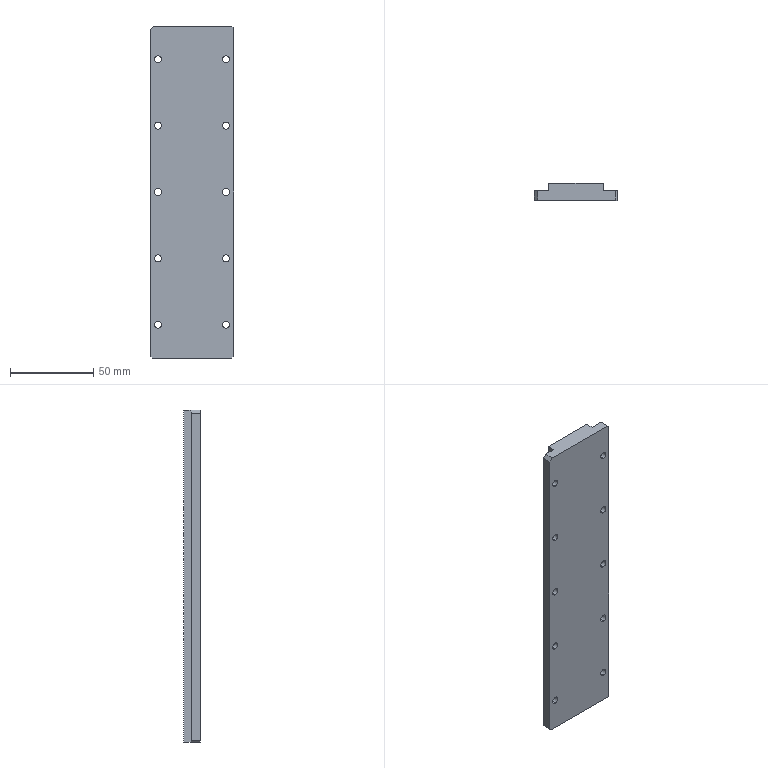Part | SolidWorks | features BaseBody 1 | 1 solid | 104 faces | box 50 x 10.1 x 200 mm | volume 84250 mm3 | plane 48 | cylinder 40 | spline 16 | commonest cylinder face diameters 4.3 x20 7.6 x20